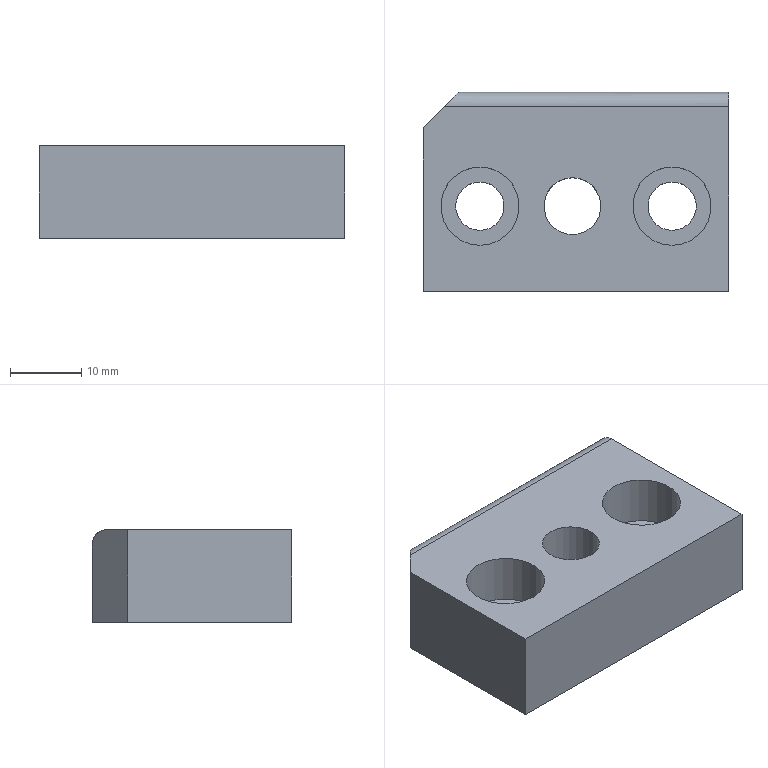Part | STEP file | gslz 2016.10.28-13_id298_x_t | 1 solid | 15 faces | box 43 x 28 x 13 mm | volume 13037 mm3 | plane 9 | cylinder 6 | commonest cylinder face diameters 6.8 x2 11 x2 4 x1 8 x1
STEP:
#1=CARTESIAN_POINT('',(0.,0.,0.));
#2=DIRECTION('',(0.,0.,1.));
#3=DIRECTION('',(1.,0.,0.));
#4=AXIS2_PLACEMENT_3D('',#1,#2,#3);
#5=CARTESIAN_POINT('',(72.5,53.692,-13.));
#6=VERTEX_POINT('',#5);
#7=CARTESIAN_POINT('',(72.5,81.692,-13.));
#8=VERTEX_POINT('',#7);
#9=CARTESIAN_POINT('',(72.5,88.142,-13.));
#10=DIRECTION('',(0.,1.,0.));
#11=VECTOR('',#10,1.);
#12=LINE('',#9,#11);
#13=CARTESIAN_POINT('',(72.5,88.142,-5.));
#14=DIRECTION('',(-1.,0.,0.));
#15=DIRECTION('',(0.,0.,-1.));
#16=AXIS2_PLACEMENT_3D('',#13,#14,#15);
#17=PLANE('',#16);
#18=CARTESIAN_POINT('',(8.,0.));
#19=DIRECTION('',(0.,-1.));
#20=VECTOR('',#19,1.);
#21=LINE('',#18,#20);
#22=(GEOMETRIC_REPRESENTATION_CONTEXT(2)PARAMETRIC_REPRESENTATION_CONTEXT()REPRESENTATION_CONTEXT('',''));
#23=DEFINITIONAL_REPRESENTATION('',(#21),#22);
#24=PCURVE('',#17,#23);
#25=CARTESIAN_POINT('',(-412.493,94.567,-13.));
#26=DIRECTION('',(0.,0.,1.));
#27=DIRECTION('',(-1.,0.,0.));
#28=AXIS2_PLACEMENT_3D('',#25,#26,#27);
#29=PLANE('',#28);
#30=CARTESIAN_POINT('',(-484.993,6.425));
#31=DIRECTION('',(0.,-1.));
#32=VECTOR('',#31,1.);
#33=LINE('',#30,#32);
#34=(GEOMETRIC_REPRESENTATION_CONTEXT(2)PARAMETRIC_REPRESENTATION_CONTEXT()REPRESENTATION_CONTEXT('',''));
#35=DEFINITIONAL_REPRESENTATION('',(#33),#34);
#36=PCURVE('',#29,#35);
#37=SURFACE_CURVE('',#12,(#24,#36),.PCURVE_S1.);
#38=EDGE_CURVE('',#6,#8,#37,.T.);
#39=ORIENTED_EDGE('',*,*,#38,.T.);
#40=CARTESIAN_POINT('',(72.5,81.692,-2.));
#41=VERTEX_POINT('',#40);
#42=CARTESIAN_POINT('',(72.5,81.692,-5.));
#43=DIRECTION('',(0.,0.,1.));
#44=VECTOR('',#43,1.);
#45=LINE('',#42,#44);
#46=CARTESIAN_POINT('',(0.,6.45));
#47=DIRECTION('',(-1.,0.));
#48=VECTOR('',#47,1.);
#49=LINE('',#46,#48);
#50=(GEOMETRIC_REPRESENTATION_CONTEXT(2)PARAMETRIC_REPRESENTATION_CONTEXT()REPRESENTATION_CONTEXT('',''));
#51=DEFINITIONAL_REPRESENTATION('',(#49),#50);
#52=PCURVE('',#17,#51);
#53=CARTESIAN_POINT('',(-39.228,81.692,-16.));
#54=DIRECTION('',(0.,-1.,0.));
#55=DIRECTION('',(0.,0.,1.));
#56=AXIS2_PLACEMENT_3D('',#53,#54,#55);
#57=PLANE('',#56);
#58=CARTESIAN_POINT('',(11.,-111.728));
#59=DIRECTION('',(1.,0.));
#60=VECTOR('',#59,1.);
#61=LINE('',#58,#60);
#62=(GEOMETRIC_REPRESENTATION_CONTEXT(2)PARAMETRIC_REPRESENTATION_CONTEXT()REPRESENTATION_CONTEXT('',''));
#63=DEFINITIONAL_REPRESENTATION('',(#61),#62);
#64=PCURVE('',#57,#63);
#65=SURFACE_CURVE('',#45,(#52,#64),.PCURVE_S1.);
#66=EDGE_CURVE('',#8,#41,#65,.T.);
#67=ORIENTED_EDGE('',*,*,#66,.T.);
#68=CARTESIAN_POINT('',(72.5,79.692,0.));
#69=VERTEX_POINT('',#68);
#70=CARTESIAN_POINT('',(72.5,79.692,-2.));
#71=DIRECTION('',(-1.,0.,0.));
#72=DIRECTION('',(0.,0.,1.));
#73=AXIS2_PLACEMENT_3D('',#70,#71,#72);
#74=CIRCLE('',#73,2.);
#75=CARTESIAN_POINT('',(-3.,8.45));
#76=DIRECTION('',(-1.,0.));
#77=AXIS2_PLACEMENT_2D('',#75,#76);
#78=CIRCLE('',#77,2.);
#79=(GEOMETRIC_REPRESENTATION_CONTEXT(2)PARAMETRIC_REPRESENTATION_CONTEXT()REPRESENTATION_CONTEXT('',''));
#80=DEFINITIONAL_REPRESENTATION('',(#78),#79);
#81=PCURVE('',#17,#80);
#82=CARTESIAN_POINT('',(-412.493,79.692,-2.));
#83=DIRECTION('',(1.,0.,0.));
#84=DIRECTION('',(0.,0.,-1.));
#85=AXIS2_PLACEMENT_3D('',#82,#83,#84);
#86=CYLINDRICAL_SURFACE('',#85,2.);
#87=CARTESIAN_POINT('',(3.142,484.993));
#88=DIRECTION('',(-1.,0.));
#89=VECTOR('',#88,1.);
#90=LINE('',#87,#89);
#91=(GEOMETRIC_REPRESENTATION_CONTEXT(2)PARAMETRIC_REPRESENTATION_CONTEXT()REPRESENTATION_CONTEXT('',''));
#92=DEFINITIONAL_REPRESENTATION('',(#90),#91);
#93=PCURVE('',#86,#92);
#94=SURFACE_CURVE('',#74,(#81,#93),.PCURVE_S1.);
#95=EDGE_CURVE('',#69,#41,#94,.T.);
#96=ORIENTED_EDGE('',*,*,#95,.F.);
#97=CARTESIAN_POINT('',(72.5,53.692,0.));
#98=VERTEX_POINT('',#97);
#99=CARTESIAN_POINT('',(72.5,88.142,0.));
#100=DIRECTION('',(0.,-1.,0.));
#101=VECTOR('',#100,1.);
#102=LINE('',#99,#101);
#103=CARTESIAN_POINT('',(-5.,0.));
#104=DIRECTION('',(0.,1.));
#105=VECTOR('',#104,1.);
#106=LINE('',#103,#105);
#107=(GEOMETRIC_REPRESENTATION_CONTEXT(2)PARAMETRIC_REPRESENTATION_CONTEXT()REPRESENTATION_CONTEXT('',''));
#108=DEFINITIONAL_REPRESENTATION('',(#106),#107);
#109=PCURVE('',#17,#108);
#110=CARTESIAN_POINT('',(-412.493,94.567,0.));
#111=DIRECTION('',(0.,0.,1.));
#112=DIRECTION('',(-1.,0.,0.));
#113=AXIS2_PLACEMENT_3D('',#110,#111,#112);
#114=PLANE('',#113);
#115=CARTESIAN_POINT('',(-484.993,6.425));
#116=DIRECTION('',(0.,1.));
#117=VECTOR('',#116,1.);
#118=LINE('',#115,#117);
#119=(GEOMETRIC_REPRESENTATION_CONTEXT(2)PARAMETRIC_REPRESENTATION_CONTEXT()REPRESENTATION_CONTEXT('',''));
#120=DEFINITIONAL_REPRESENTATION('',(#118),#119);
#121=PCURVE('',#114,#120);
#122=SURFACE_CURVE('',#102,(#109,#121),.PCURVE_S1.);
#123=EDGE_CURVE('',#69,#98,#122,.T.);
#124=ORIENTED_EDGE('',*,*,#123,.T.);
#125=CARTESIAN_POINT('',(72.5,53.692,-16.));
#126=DIRECTION('',(0.,0.,-1.));
#127=VECTOR('',#126,1.);
#128=LINE('',#125,#127);
#129=CARTESIAN_POINT('',(11.,34.45));
#130=DIRECTION('',(1.,0.));
#131=VECTOR('',#130,1.);
#132=LINE('',#129,#131);
#133=(GEOMETRIC_REPRESENTATION_CONTEXT(2)PARAMETRIC_REPRESENTATION_CONTEXT()REPRESENTATION_CONTEXT('',''));
#134=DEFINITIONAL_REPRESENTATION('',(#132),#133);
#135=PCURVE('',#17,#134);
#136=CARTESIAN_POINT('',(-39.228,53.692,-16.));
#137=DIRECTION('',(0.,-1.,0.));
#138=DIRECTION('',(0.,0.,1.));
#139=AXIS2_PLACEMENT_3D('',#136,#137,#138);
#140=PLANE('',#139);
#141=CARTESIAN_POINT('',(0.,-111.728));
#142=DIRECTION('',(-1.,0.));
#143=VECTOR('',#142,1.);
#144=LINE('',#141,#143);
#145=(GEOMETRIC_REPRESENTATION_CONTEXT(2)PARAMETRIC_REPRESENTATION_CONTEXT()REPRESENTATION_CONTEXT('',''));
#146=DEFINITIONAL_REPRESENTATION('',(#144),#145);
#147=PCURVE('',#140,#146);
#148=SURFACE_CURVE('',#128,(#135,#147),.PCURVE_S1.);
#149=EDGE_CURVE('',#98,#6,#148,.T.);
#150=ORIENTED_EDGE('',*,*,#149,.T.);
#151=EDGE_LOOP('',(#39,#67,#96,#124,#150));
#152=FACE_BOUND('',#151,.T.);
#153=ADVANCED_FACE('',(#152),#17,.F.);
#154=CARTESIAN_POINT('',(29.5,53.692,0.));
#155=VERTEX_POINT('',#154);
#156=CARTESIAN_POINT('',(29.5,76.692,0.));
#157=VERTEX_POINT('',#156);
#158=CARTESIAN_POINT('',(29.5,88.142,0.));
#159=DIRECTION('',(0.,1.,0.));
#160=VECTOR('',#159,1.);
#161=LINE('',#158,#160);
#162=CARTESIAN_POINT('',(29.5,88.142,-5.));
#163=DIRECTION('',(-1.,0.,0.));
#164=DIRECTION('',(0.,0.,-1.));
#165=AXIS2_PLACEMENT_3D('',#162,#163,#164);
#166=PLANE('',#165);
#167=CARTESIAN_POINT('',(-5.,0.));
#168=DIRECTION('',(0.,-1.));
#169=VECTOR('',#168,1.);
#170=LINE('',#167,#169);
#171=(GEOMETRIC_REPRESENTATION_CONTEXT(2)PARAMETRIC_REPRESENTATION_CONTEXT()REPRESENTATION_CONTEXT('',''));
#172=DEFINITIONAL_REPRESENTATION('',(#170),#171);
#173=PCURVE('',#166,#172);
#174=CARTESIAN_POINT('',(-441.993,6.425));
#175=DIRECTION('',(0.,-1.));
#176=VECTOR('',#175,1.);
#177=LINE('',#174,#176);
#178=(GEOMETRIC_REPRESENTATION_CONTEXT(2)PARAMETRIC_REPRESENTATION_CONTEXT()REPRESENTATION_CONTEXT('',''));
#179=DEFINITIONAL_REPRESENTATION('',(#177),#178);
#180=PCURVE('',#114,#179);
#181=SURFACE_CURVE('',#161,(#173,#180),.PCURVE_S1.);
#182=EDGE_CURVE('',#155,#157,#181,.T.);
#183=ORIENTED_EDGE('',*,*,#182,.T.);
#184=CARTESIAN_POINT('',(29.5,76.692,-13.));
#185=VERTEX_POINT('',#184);
#186=CARTESIAN_POINT('',(29.5,76.692,-5.));
#187=DIRECTION('',(0.,0.,-1.));
#188=VECTOR('',#187,1.);
#189=LINE('',#186,#188);
#190=CARTESIAN_POINT('',(0.,11.45));
#191=DIRECTION('',(1.,0.));
#192=VECTOR('',#191,1.);
#193=LINE('',#190,#192);
#194=(GEOMETRIC_REPRESENTATION_CONTEXT(2)PARAMETRIC_REPRESENTATION_CONTEXT()REPRESENTATION_CONTEXT('',''));
#195=DEFINITIONAL_REPRESENTATION('',(#193),#194);
#196=PCURVE('',#166,#195);
#197=CARTESIAN_POINT('',(34.5,81.692,-16.));
#198=DIRECTION('',(-0.7071,0.7071,0.));
#199=DIRECTION('',(-0.7071,-0.7071,0.));
#200=AXIS2_PLACEMENT_3D('',#197,#198,#199);
#201=PLANE('',#200);
#202=CARTESIAN_POINT('',(7.071,11.));
#203=DIRECTION('',(0.,-1.));
#204=VECTOR('',#203,1.);
#205=LINE('',#202,#204);
#206=(GEOMETRIC_REPRESENTATION_CONTEXT(2)PARAMETRIC_REPRESENTATION_CONTEXT()REPRESENTATION_CONTEXT('',''));
#207=DEFINITIONAL_REPRESENTATION('',(#205),#206);
#208=PCURVE('',#201,#207);
#209=SURFACE_CURVE('',#189,(#196,#208),.PCURVE_S1.);
#210=EDGE_CURVE('',#157,#185,#209,.T.);
#211=ORIENTED_EDGE('',*,*,#210,.T.);
#212=CARTESIAN_POINT('',(29.5,53.692,-13.));
#213=VERTEX_POINT('',#212);
#214=CARTESIAN_POINT('',(29.5,88.142,-13.));
#215=DIRECTION('',(0.,-1.,0.));
#216=VECTOR('',#215,1.);
#217=LINE('',#214,#216);
#218=CARTESIAN_POINT('',(8.,0.));
#219=DIRECTION('',(0.,1.));
#220=VECTOR('',#219,1.);
#221=LINE('',#218,#220);
#222=(GEOMETRIC_REPRESENTATION_CONTEXT(2)PARAMETRIC_REPRESENTATION_CONTEXT()REPRESENTATION_CONTEXT('',''));
#223=DEFINITIONAL_REPRESENTATION('',(#221),#222);
#224=PCURVE('',#166,#223);
#225=CARTESIAN_POINT('',(-441.993,6.425));
#226=DIRECTION('',(0.,1.));
#227=VECTOR('',#226,1.);
#228=LINE('',#225,#227);
#229=(GEOMETRIC_REPRESENTATION_CONTEXT(2)PARAMETRIC_REPRESENTATION_CONTEXT()REPRESENTATION_CONTEXT('',''));
#230=DEFINITIONAL_REPRESENTATION('',(#228),#229);
#231=PCURVE('',#29,#230);
#232=SURFACE_CURVE('',#217,(#224,#231),.PCURVE_S1.);
#233=EDGE_CURVE('',#185,#213,#232,.T.);
#234=ORIENTED_EDGE('',*,*,#233,.T.);
#235=CARTESIAN_POINT('',(29.5,53.692,-5.));
#236=DIRECTION('',(0.,0.,-1.));
#237=VECTOR('',#236,1.);
#238=LINE('',#235,#237);
#239=CARTESIAN_POINT('',(0.,34.45));
#240=DIRECTION('',(1.,0.));
#241=VECTOR('',#240,1.);
#242=LINE('',#239,#241);
#243=(GEOMETRIC_REPRESENTATION_CONTEXT(2)PARAMETRIC_REPRESENTATION_CONTEXT()REPRESENTATION_CONTEXT('',''));
#244=DEFINITIONAL_REPRESENTATION('',(#242),#243);
#245=PCURVE('',#166,#244);
#246=CARTESIAN_POINT('',(11.,-68.728));
#247=DIRECTION('',(-1.,0.));
#248=VECTOR('',#247,1.);
#249=LINE('',#246,#248);
#250=(GEOMETRIC_REPRESENTATION_CONTEXT(2)PARAMETRIC_REPRESENTATION_CONTEXT()REPRESENTATION_CONTEXT('',''));
#251=DEFINITIONAL_REPRESENTATION('',(#249),#250);
#252=PCURVE('',#140,#251);
#253=SURFACE_CURVE('',#238,(#245,#252),.PCURVE_S1.);
#254=EDGE_CURVE('',#155,#213,#253,.T.);
#255=ORIENTED_EDGE('',*,*,#254,.F.);
#256=EDGE_LOOP('',(#183,#211,#234,#255));
#257=FACE_BOUND('',#256,.T.);
#258=ADVANCED_FACE('',(#257),#166,.T.);
#259=CARTESIAN_POINT('',(64.5,60.192,0.));
#260=VERTEX_POINT('',#259);
#261=CARTESIAN_POINT('',(64.5,65.692,0.));
#262=DIRECTION('',(0.,0.,-1.));
#263=DIRECTION('',(0.,-1.,0.));
#264=AXIS2_PLACEMENT_3D('',#261,#262,#263);
#265=CIRCLE('',#264,5.5);
#266=CARTESIAN_POINT('',(-476.993,34.375));
#267=CARTESIAN_POINT('',(-467.467,34.375));
#268=CARTESIAN_POINT('',(-472.23,26.125));
#269=CARTESIAN_POINT('',(-476.993,17.875));
#270=CARTESIAN_POINT('',(-481.756,26.125));
#271=CARTESIAN_POINT('',(-486.519,34.375));
#272=CARTESIAN_POINT('',(-476.993,34.375));
#273=(BOUNDED_CURVE()B_SPLINE_CURVE(2,(#266,#267,#268,#269,#270,#271,#272),.UNSPECIFIED.,.T.,.F.)B_SPLINE_CURVE_WITH_KNOTS((1,2,2,2,2,1),(-2.094,0.,2.094,4.189,6.283,8.378),.UNSPECIFIED.)CURVE()GEOMETRIC_REPRESENTATION_ITEM()RATIONAL_B_SPLINE_CURVE((1.,0.5,1.,0.5,1.,0.5,1.))REPRESENTATION_ITEM(''));
#274=(GEOMETRIC_REPRESENTATION_CONTEXT(2)PARAMETRIC_REPRESENTATION_CONTEXT()REPRESENTATION_CONTEXT('',''));
#275=DEFINITIONAL_REPRESENTATION('',(#273),#274);
#276=PCURVE('',#114,#275);
#277=CARTESIAN_POINT('',(64.5,65.692,0.));
#278=DIRECTION('',(0.,0.,-1.));
#279=DIRECTION('',(0.,-1.,0.));
#280=AXIS2_PLACEMENT_3D('',#277,#278,#279);
#281=CYLINDRICAL_SURFACE('',#280,5.5);
#282=CARTESIAN_POINT('',(0.,0.));
#283=DIRECTION('',(1.,0.));
#284=VECTOR('',#283,1.);
#285=LINE('',#282,#284);
#286=(GEOMETRIC_REPRESENTATION_CONTEXT(2)PARAMETRIC_REPRESENTATION_CONTEXT()REPRESENTATION_CONTEXT('',''));
#287=DEFINITIONAL_REPRESENTATION('',(#285),#286);
#288=PCURVE('',#281,#287);
#289=SURFACE_CURVE('',#265,(#276,#288),.PCURVE_S1.);
#290=EDGE_CURVE('',#260,#260,#289,.T.);
#291=ORIENTED_EDGE('',*,*,#290,.T.);
#292=EDGE_LOOP('',(#291));
#293=FACE_BOUND('',#292,.T.);
#294=CARTESIAN_POINT('',(37.5,60.192,0.));
#295=VERTEX_POINT('',#294);
#296=CARTESIAN_POINT('',(37.5,65.692,0.));
#297=DIRECTION('',(0.,0.,-1.));
#298=DIRECTION('',(0.,-1.,0.));
#299=AXIS2_PLACEMENT_3D('',#296,#297,#298);
#300=CIRCLE('',#299,5.5);
#301=CARTESIAN_POINT('',(-449.993,34.375));
#302=CARTESIAN_POINT('',(-440.467,34.375));
#303=CARTESIAN_POINT('',(-445.23,26.125));
#304=CARTESIAN_POINT('',(-449.993,17.875));
#305=CARTESIAN_POINT('',(-454.756,26.125));
#306=CARTESIAN_POINT('',(-459.519,34.375));
#307=CARTESIAN_POINT('',(-449.993,34.375));
#308=(BOUNDED_CURVE()B_SPLINE_CURVE(2,(#301,#302,#303,#304,#305,#306,#307),.UNSPECIFIED.,.T.,.F.)B_SPLINE_CURVE_WITH_KNOTS((1,2,2,2,2,1),(-2.094,0.,2.094,4.189,6.283,8.378),.UNSPECIFIED.)CURVE()GEOMETRIC_REPRESENTATION_ITEM()RATIONAL_B_SPLINE_CURVE((1.,0.5,1.,0.5,1.,0.5,1.))REPRESENTATION_ITEM(''));
#309=(GEOMETRIC_REPRESENTATION_CONTEXT(2)PARAMETRIC_REPRESENTATION_CONTEXT()REPRESENTATION_CONTEXT('',''));
#310=DEFINITIONAL_REPRESENTATION('',(#308),#309);
#311=PCURVE('',#114,#310);
#312=CARTESIAN_POINT('',(37.5,65.692,0.));
#313=DIRECTION('',(0.,0.,-1.));
#314=DIRECTION('',(0.,-1.,0.));
#315=AXIS2_PLACEMENT_3D('',#312,#313,#314);
#316=CYLINDRICAL_SURFACE('',#315,5.5);
#317=CARTESIAN_POINT('',(0.,0.));
#318=DIRECTION('',(1.,0.));
#319=VECTOR('',#318,1.);
#320=LINE('',#317,#319);
#321=(GEOMETRIC_REPRESENTATION_CONTEXT(2)PARAMETRIC_REPRESENTATION_CONTEXT()REPRESENTATION_CONTEXT('',''));
#322=DEFINITIONAL_REPRESENTATION('',(#320),#321);
#323=PCURVE('',#316,#322);
#324=SURFACE_CURVE('',#300,(#311,#323),.PCURVE_S1.);
#325=EDGE_CURVE('',#295,#295,#324,.T.);
#326=ORIENTED_EDGE('',*,*,#325,.T.);
#327=EDGE_LOOP('',(#326));
#328=FACE_BOUND('',#327,.T.);
#329=CARTESIAN_POINT('',(50.5,61.692,0.));
#330=VERTEX_POINT('',#329);
#331=CARTESIAN_POINT('',(50.5,65.692,0.));
#332=DIRECTION('',(0.,0.,1.));
#333=DIRECTION('',(0.,-1.,0.));
#334=AXIS2_PLACEMENT_3D('',#331,#332,#333);
#335=CIRCLE('',#334,4.);
#336=CARTESIAN_POINT('',(-462.993,28.875));
#337=DIRECTION('',(0.,1.));
#338=AXIS2_PLACEMENT_2D('',#336,#337);
#339=CIRCLE('',#338,4.);
#340=(GEOMETRIC_REPRESENTATION_CONTEXT(2)PARAMETRIC_REPRESENTATION_CONTEXT()REPRESENTATION_CONTEXT('',''));
#341=DEFINITIONAL_REPRESENTATION('',(#339),#340);
#342=PCURVE('',#114,#341);
#343=CARTESIAN_POINT('',(50.5,65.692,-50.));
#344=DIRECTION('',(0.,0.,-1.));
#345=DIRECTION('',(0.,-1.,0.));
#346=AXIS2_PLACEMENT_3D('',#343,#344,#345);
#347=CYLINDRICAL_SURFACE('',#346,4.);
#348=CARTESIAN_POINT('',(6.283,-50.));
#349=DIRECTION('',(-1.,0.));
#350=VECTOR('',#349,1.);
#351=LINE('',#348,#350);
#352=(GEOMETRIC_REPRESENTATION_CONTEXT(2)PARAMETRIC_REPRESENTATION_CONTEXT()REPRESENTATION_CONTEXT('',''));
#353=DEFINITIONAL_REPRESENTATION('',(#351),#352);
#354=PCURVE('',#347,#353);
#355=SURFACE_CURVE('',#335,(#342,#354),.PCURVE_S1.);
#356=EDGE_CURVE('',#330,#330,#355,.T.);
#357=ORIENTED_EDGE('',*,*,#356,.F.);
#358=EDGE_LOOP('',(#357));
#359=FACE_BOUND('',#358,.T.);
#360=ORIENTED_EDGE('',*,*,#123,.F.);
#361=CARTESIAN_POINT('',(32.5,79.692,0.));
#362=VERTEX_POINT('',#361);
#363=CARTESIAN_POINT('',(-412.493,79.692,0.));
#364=DIRECTION('',(-1.,0.,0.));
#365=VECTOR('',#364,1.);
#366=LINE('',#363,#365);
#367=CARTESIAN_POINT('',(0.,14.875));
#368=DIRECTION('',(1.,0.));
#369=VECTOR('',#368,1.);
#370=LINE('',#367,#369);
#371=(GEOMETRIC_REPRESENTATION_CONTEXT(2)PARAMETRIC_REPRESENTATION_CONTEXT()REPRESENTATION_CONTEXT('',''));
#372=DEFINITIONAL_REPRESENTATION('',(#370),#371);
#373=PCURVE('',#114,#372);
#374=CARTESIAN_POINT('',(3.142,0.));
#375=DIRECTION('',(0.,-1.));
#376=VECTOR('',#375,1.);
#377=LINE('',#374,#376);
#378=(GEOMETRIC_REPRESENTATION_CONTEXT(2)PARAMETRIC_REPRESENTATION_CONTEXT()REPRESENTATION_CONTEXT('',''));
#379=DEFINITIONAL_REPRESENTATION('',(#377),#378);
#380=PCURVE('',#86,#379);
#381=SURFACE_CURVE('',#366,(#373,#380),.PCURVE_S1.);
#382=EDGE_CURVE('',#69,#362,#381,.T.);
#383=ORIENTED_EDGE('',*,*,#382,.T.);
#384=CARTESIAN_POINT('',(-182.559,-135.367,0.));
#385=DIRECTION('',(-0.7071,-0.7071,0.));
#386=VECTOR('',#385,1.);
#387=LINE('',#384,#386);
#388=CARTESIAN_POINT('',(-229.934,229.934));
#389=DIRECTION('',(0.7071,0.7071));
#390=VECTOR('',#389,1.);
#391=LINE('',#388,#390);
#392=(GEOMETRIC_REPRESENTATION_CONTEXT(2)PARAMETRIC_REPRESENTATION_CONTEXT()REPRESENTATION_CONTEXT('',''));
#393=DEFINITIONAL_REPRESENTATION('',(#391),#392);
#394=PCURVE('',#114,#393);
#395=CARTESIAN_POINT('',(306.968,16.));
#396=DIRECTION('',(1.,0.));
#397=VECTOR('',#396,1.);
#398=LINE('',#395,#397);
#399=(GEOMETRIC_REPRESENTATION_CONTEXT(2)PARAMETRIC_REPRESENTATION_CONTEXT()REPRESENTATION_CONTEXT('',''));
#400=DEFINITIONAL_REPRESENTATION('',(#398),#399);
#401=PCURVE('',#201,#400);
#402=SURFACE_CURVE('',#387,(#394,#401),.PCURVE_S1.);
#403=EDGE_CURVE('',#362,#157,#402,.T.);
#404=ORIENTED_EDGE('',*,*,#403,.T.);
#405=ORIENTED_EDGE('',*,*,#182,.F.);
#406=CARTESIAN_POINT('',(-39.228,53.692,0.));
#407=DIRECTION('',(-1.,0.,0.));
#408=VECTOR('',#407,1.);
#409=LINE('',#406,#408);
#410=CARTESIAN_POINT('',(-373.265,40.875));
#411=DIRECTION('',(1.,0.));
#412=VECTOR('',#411,1.);
#413=LINE('',#410,#412);
#414=(GEOMETRIC_REPRESENTATION_CONTEXT(2)PARAMETRIC_REPRESENTATION_CONTEXT()REPRESENTATION_CONTEXT('',''));
#415=DEFINITIONAL_REPRESENTATION('',(#413),#414);
#416=PCURVE('',#114,#415);
#417=CARTESIAN_POINT('',(16.,0.));
#418=DIRECTION('',(0.,1.));
#419=VECTOR('',#418,1.);
#420=LINE('',#417,#419);
#421=(GEOMETRIC_REPRESENTATION_CONTEXT(2)PARAMETRIC_REPRESENTATION_CONTEXT()REPRESENTATION_CONTEXT('',''));
#422=DEFINITIONAL_REPRESENTATION('',(#420),#421);
#423=PCURVE('',#140,#422);
#424=SURFACE_CURVE('',#409,(#416,#423),.PCURVE_S1.);
#425=EDGE_CURVE('',#98,#155,#424,.T.);
#426=ORIENTED_EDGE('',*,*,#425,.F.);
#427=EDGE_LOOP('',(#360,#383,#404,#405,#426));
#428=FACE_BOUND('',#427,.T.);
#429=ADVANCED_FACE('',(#293,#328,#359,#428),#114,.T.);
#430=CARTESIAN_POINT('',(64.5,62.292,-13.));
#431=VERTEX_POINT('',#430);
#432=CARTESIAN_POINT('',(64.5,65.692,-13.));
#433=DIRECTION('',(0.,0.,-1.));
#434=DIRECTION('',(0.,-1.,0.));
#435=AXIS2_PLACEMENT_3D('',#432,#433,#434);
#436=CIRCLE('',#435,3.4);
#437=CARTESIAN_POINT('',(-476.993,32.275));
#438=CARTESIAN_POINT('',(-471.104,32.275));
#439=CARTESIAN_POINT('',(-474.048,27.175));
#440=CARTESIAN_POINT('',(-476.993,22.075));
#441=CARTESIAN_POINT('',(-479.937,27.175));
#442=CARTESIAN_POINT('',(-482.882,32.275));
#443=CARTESIAN_POINT('',(-476.993,32.275));
#444=(BOUNDED_CURVE()B_SPLINE_CURVE(2,(#437,#438,#439,#440,#441,#442,#443),.UNSPECIFIED.,.T.,.F.)B_SPLINE_CURVE_WITH_KNOTS((1,2,2,2,2,1),(-2.094,0.,2.094,4.189,6.283,8.378),.UNSPECIFIED.)CURVE()GEOMETRIC_REPRESENTATION_ITEM()RATIONAL_B_SPLINE_CURVE((1.,0.5,1.,0.5,1.,0.5,1.))REPRESENTATION_ITEM(''));
#445=(GEOMETRIC_REPRESENTATION_CONTEXT(2)PARAMETRIC_REPRESENTATION_CONTEXT()REPRESENTATION_CONTEXT('',''));
#446=DEFINITIONAL_REPRESENTATION('',(#444),#445);
#447=PCURVE('',#29,#446);
#448=CARTESIAN_POINT('',(64.5,65.692,-50.));
#449=DIRECTION('',(0.,0.,-1.));
#450=DIRECTION('',(0.,-1.,0.));
#451=AXIS2_PLACEMENT_3D('',#448,#449,#450);
#452=CYLINDRICAL_SURFACE('',#451,3.4);
#453=CARTESIAN_POINT('',(0.,-37.));
#454=DIRECTION('',(1.,0.));
#455=VECTOR('',#454,1.);
#456=LINE('',#453,#455);
#457=(GEOMETRIC_REPRESENTATION_CONTEXT(2)PARAMETRIC_REPRESENTATION_CONTEXT()REPRESENTATION_CONTEXT('',''));
#458=DEFINITIONAL_REPRESENTATION('',(#456),#457);
#459=PCURVE('',#452,#458);
#460=SURFACE_CURVE('',#436,(#447,#459),.PCURVE_S1.);
#461=EDGE_CURVE('',#431,#431,#460,.T.);
#462=ORIENTED_EDGE('',*,*,#461,.F.);
#463=EDGE_LOOP('',(#462));
#464=FACE_BOUND('',#463,.T.);
#465=CARTESIAN_POINT('',(37.5,62.292,-13.));
#466=VERTEX_POINT('',#465);
#467=CARTESIAN_POINT('',(37.5,65.692,-13.));
#468=DIRECTION('',(0.,0.,-1.));
#469=DIRECTION('',(0.,-1.,0.));
#470=AXIS2_PLACEMENT_3D('',#467,#468,#469);
#471=CIRCLE('',#470,3.4);
#472=CARTESIAN_POINT('',(-449.993,32.275));
#473=CARTESIAN_POINT('',(-444.104,32.275));
#474=CARTESIAN_POINT('',(-447.048,27.175));
#475=CARTESIAN_POINT('',(-449.993,22.075));
#476=CARTESIAN_POINT('',(-452.937,27.175));
#477=CARTESIAN_POINT('',(-455.882,32.275));
#478=CARTESIAN_POINT('',(-449.993,32.275));
#479=(BOUNDED_CURVE()B_SPLINE_CURVE(2,(#472,#473,#474,#475,#476,#477,#478),.UNSPECIFIED.,.T.,.F.)B_SPLINE_CURVE_WITH_KNOTS((1,2,2,2,2,1),(-2.094,0.,2.094,4.189,6.283,8.378),.UNSPECIFIED.)CURVE()GEOMETRIC_REPRESENTATION_ITEM()RATIONAL_B_SPLINE_CURVE((1.,0.5,1.,0.5,1.,0.5,1.))REPRESENTATION_ITEM(''));
#480=(GEOMETRIC_REPRESENTATION_CONTEXT(2)PARAMETRIC_REPRESENTATION_CONTEXT()REPRESENTATION_CONTEXT('',''));
#481=DEFINITIONAL_REPRESENTATION('',(#479),#480);
#482=PCURVE('',#29,#481);
#483=CARTESIAN_POINT('',(37.5,65.692,-50.));
#484=DIRECTION('',(0.,0.,-1.));
#485=DIRECTION('',(0.,-1.,0.));
#486=AXIS2_PLACEMENT_3D('',#483,#484,#485);
#487=CYLINDRICAL_SURFACE('',#486,3.4);
#488=CARTESIAN_POINT('',(0.,-37.));
#489=DIRECTION('',(1.,0.));
#490=VECTOR('',#489,1.);
#491=LINE('',#488,#490);
#492=(GEOMETRIC_REPRESENTATION_CONTEXT(2)PARAMETRIC_REPRESENTATION_CONTEXT()REPRESENTATION_CONTEXT('',''));
#493=DEFINITIONAL_REPRESENTATION('',(#491),#492);
#494=PCURVE('',#487,#493);
#495=SURFACE_CURVE('',#471,(#482,#494),.PCURVE_S1.);
#496=EDGE_CURVE('',#466,#466,#495,.T.);
#497=ORIENTED_EDGE('',*,*,#496,.F.);
#498=EDGE_LOOP('',(#497));
#499=FACE_BOUND('',#498,.T.);
#500=CARTESIAN_POINT('',(50.5,61.692,-13.));
#501=VERTEX_POINT('',#500);
#502=CARTESIAN_POINT('',(50.5,65.692,-13.));
#503=DIRECTION('',(0.,0.,-1.));
#504=DIRECTION('',(0.,-1.,0.));
#505=AXIS2_PLACEMENT_3D('',#502,#503,#504);
#506=CIRCLE('',#505,4.);
#507=CARTESIAN_POINT('',(-462.993,32.875));
#508=CARTESIAN_POINT('',(-456.065,32.875));
#509=CARTESIAN_POINT('',(-459.529,26.875));
#510=CARTESIAN_POINT('',(-462.993,20.875));
#511=CARTESIAN_POINT('',(-466.457,26.875));
#512=CARTESIAN_POINT('',(-469.921,32.875));
#513=CARTESIAN_POINT('',(-462.993,32.875));
#514=(BOUNDED_CURVE()B_SPLINE_CURVE(2,(#507,#508,#509,#510,#511,#512,#513),.UNSPECIFIED.,.T.,.F.)B_SPLINE_CURVE_WITH_KNOTS((1,2,2,2,2,1),(-2.094,0.,2.094,4.189,6.283,8.378),.UNSPECIFIED.)CURVE()GEOMETRIC_REPRESENTATION_ITEM()RATIONAL_B_SPLINE_CURVE((1.,0.5,1.,0.5,1.,0.5,1.))REPRESENTATION_ITEM(''));
#515=(GEOMETRIC_REPRESENTATION_CONTEXT(2)PARAMETRIC_REPRESENTATION_CONTEXT()REPRESENTATION_CONTEXT('',''));
#516=DEFINITIONAL_REPRESENTATION('',(#514),#515);
#517=PCURVE('',#29,#516);
#518=CARTESIAN_POINT('',(0.,-37.));
#519=DIRECTION('',(1.,0.));
#520=VECTOR('',#519,1.);
#521=LINE('',#518,#520);
#522=(GEOMETRIC_REPRESENTATION_CONTEXT(2)PARAMETRIC_REPRESENTATION_CONTEXT()REPRESENTATION_CONTEXT('',''));
#523=DEFINITIONAL_REPRESENTATION('',(#521),#522);
#524=PCURVE('',#347,#523);
#525=SURFACE_CURVE('',#506,(#517,#524),.PCURVE_S1.);
#526=EDGE_CURVE('',#501,#501,#525,.T.);
#527=ORIENTED_EDGE('',*,*,#526,.F.);
#528=EDGE_LOOP('',(#527));
#529=FACE_BOUND('',#528,.T.);
#530=ORIENTED_EDGE('',*,*,#233,.F.);
#531=CARTESIAN_POINT('',(34.5,81.692,-13.));
#532=VERTEX_POINT('',#531);
#533=CARTESIAN_POINT('',(-182.559,-135.367,-13.));
#534=DIRECTION('',(0.7071,0.7071,0.));
#535=VECTOR('',#534,1.);
#536=LINE('',#533,#535);
#537=CARTESIAN_POINT('',(-229.934,229.934));
#538=DIRECTION('',(-0.7071,-0.7071));
#539=VECTOR('',#538,1.);
#540=LINE('',#537,#539);
#541=(GEOMETRIC_REPRESENTATION_CONTEXT(2)PARAMETRIC_REPRESENTATION_CONTEXT()REPRESENTATION_CONTEXT('',''));
#542=DEFINITIONAL_REPRESENTATION('',(#540),#541);
#543=PCURVE('',#29,#542);
#544=CARTESIAN_POINT('',(306.968,3.));
#545=DIRECTION('',(-1.,0.));
#546=VECTOR('',#545,1.);
#547=LINE('',#544,#546);
#548=(GEOMETRIC_REPRESENTATION_CONTEXT(2)PARAMETRIC_REPRESENTATION_CONTEXT()REPRESENTATION_CONTEXT('',''));
#549=DEFINITIONAL_REPRESENTATION('',(#547),#548);
#550=PCURVE('',#201,#549);
#551=SURFACE_CURVE('',#536,(#543,#550),.PCURVE_S1.);
#552=EDGE_CURVE('',#185,#532,#551,.T.);
#553=ORIENTED_EDGE('',*,*,#552,.T.);
#554=CARTESIAN_POINT('',(-39.228,81.692,-13.));
#555=DIRECTION('',(-1.,0.,0.));
#556=VECTOR('',#555,1.);
#557=LINE('',#554,#556);
#558=CARTESIAN_POINT('',(-373.265,12.875));
#559=DIRECTION('',(1.,0.));
#560=VECTOR('',#559,1.);
#561=LINE('',#558,#560);
#562=(GEOMETRIC_REPRESENTATION_CONTEXT(2)PARAMETRIC_REPRESENTATION_CONTEXT()REPRESENTATION_CONTEXT('',''));
#563=DEFINITIONAL_REPRESENTATION('',(#561),#562);
#564=PCURVE('',#29,#563);
#565=CARTESIAN_POINT('',(3.,0.));
#566=DIRECTION('',(0.,1.));
#567=VECTOR('',#566,1.);
#568=LINE('',#565,#567);
#569=(GEOMETRIC_REPRESENTATION_CONTEXT(2)PARAMETRIC_REPRESENTATION_CONTEXT()REPRESENTATION_CONTEXT('',''));
#570=DEFINITIONAL_REPRESENTATION('',(#568),#569);
#571=PCURVE('',#57,#570);
#572=SURFACE_CURVE('',#557,(#564,#571),.PCURVE_S1.);
#573=EDGE_CURVE('',#8,#532,#572,.T.);
#574=ORIENTED_EDGE('',*,*,#573,.F.);
#575=ORIENTED_EDGE('',*,*,#38,.F.);
#576=CARTESIAN_POINT('',(-39.228,53.692,-13.));
#577=DIRECTION('',(1.,0.,0.));
#578=VECTOR('',#577,1.);
#579=LINE('',#576,#578);
#580=CARTESIAN_POINT('',(-373.265,40.875));
#581=DIRECTION('',(-1.,0.));
#582=VECTOR('',#581,1.);
#583=LINE('',#580,#582);
#584=(GEOMETRIC_REPRESENTATION_CONTEXT(2)PARAMETRIC_REPRESENTATION_CONTEXT()REPRESENTATION_CONTEXT('',''));
#585=DEFINITIONAL_REPRESENTATION('',(#583),#584);
#586=PCURVE('',#29,#585);
#587=CARTESIAN_POINT('',(3.,0.));
#588=DIRECTION('',(0.,-1.));
#589=VECTOR('',#588,1.);
#590=LINE('',#587,#589);
#591=(GEOMETRIC_REPRESENTATION_CONTEXT(2)PARAMETRIC_REPRESENTATION_CONTEXT()REPRESENTATION_CONTEXT('',''));
#592=DEFINITIONAL_REPRESENTATION('',(#590),#591);
#593=PCURVE('',#140,#592);
#594=SURFACE_CURVE('',#579,(#586,#593),.PCURVE_S1.);
#595=EDGE_CURVE('',#213,#6,#594,.T.);
#596=ORIENTED_EDGE('',*,*,#595,.F.);
#597=EDGE_LOOP('',(#530,#553,#574,#575,#596));
#598=FACE_BOUND('',#597,.T.);
#599=ADVANCED_FACE('',(#464,#499,#529,#598),#29,.F.);
#600=CARTESIAN_POINT('',(64.5,62.292,-7.));
#601=VERTEX_POINT('',#600);
#602=CARTESIAN_POINT('',(64.5,65.692,-7.));
#603=DIRECTION('',(0.,0.,1.));
#604=DIRECTION('',(0.,-1.,0.));
#605=AXIS2_PLACEMENT_3D('',#602,#603,#604);
#606=CIRCLE('',#605,3.4);
#607=CARTESIAN_POINT('',(-412.493,94.567,-7.));
#608=DIRECTION('',(0.,0.,1.));
#609=DIRECTION('',(-1.,0.,0.));
#610=AXIS2_PLACEMENT_3D('',#607,#608,#609);
#611=PLANE('',#610);
#612=CARTESIAN_POINT('',(-476.993,28.875));
#613=DIRECTION('',(0.,1.));
#614=AXIS2_PLACEMENT_2D('',#612,#613);
#615=CIRCLE('',#614,3.4);
#616=(GEOMETRIC_REPRESENTATION_CONTEXT(2)PARAMETRIC_REPRESENTATION_CONTEXT()REPRESENTATION_CONTEXT('',''));
#617=DEFINITIONAL_REPRESENTATION('',(#615),#616);
#618=PCURVE('',#611,#617);
#619=CARTESIAN_POINT('',(6.283,-43.));
#620=DIRECTION('',(-1.,0.));
#621=VECTOR('',#620,1.);
#622=LINE('',#619,#621);
#623=(GEOMETRIC_REPRESENTATION_CONTEXT(2)PARAMETRIC_REPRESENTATION_CONTEXT()REPRESENTATION_CONTEXT('',''));
#624=DEFINITIONAL_REPRESENTATION('',(#622),#623);
#625=PCURVE('',#452,#624);
#626=SURFACE_CURVE('',#606,(#618,#625),.PCURVE_S1.);
#627=EDGE_CURVE('',#601,#601,#626,.T.);
#628=ORIENTED_EDGE('',*,*,#627,.F.);
#629=EDGE_LOOP('',(#628));
#630=FACE_BOUND('',#629,.T.);
#631=CARTESIAN_POINT('',(64.5,60.192,-7.));
#632=VERTEX_POINT('',#631);
#633=CARTESIAN_POINT('',(64.5,65.692,-7.));
#634=DIRECTION('',(0.,0.,1.));
#635=DIRECTION('',(0.,-1.,0.));
#636=AXIS2_PLACEMENT_3D('',#633,#634,#635);
#637=CIRCLE('',#636,5.5);
#638=CARTESIAN_POINT('',(-476.993,28.875));
#639=DIRECTION('',(0.,1.));
#640=AXIS2_PLACEMENT_2D('',#638,#639);
#641=CIRCLE('',#640,5.5);
#642=(GEOMETRIC_REPRESENTATION_CONTEXT(2)PARAMETRIC_REPRESENTATION_CONTEXT()REPRESENTATION_CONTEXT('',''));
#643=DEFINITIONAL_REPRESENTATION('',(#641),#642);
#644=PCURVE('',#611,#643);
#645=CARTESIAN_POINT('',(6.283,7.));
#646=DIRECTION('',(-1.,0.));
#647=VECTOR('',#646,1.);
#648=LINE('',#645,#647);
#649=(GEOMETRIC_REPRESENTATION_CONTEXT(2)PARAMETRIC_REPRESENTATION_CONTEXT()REPRESENTATION_CONTEXT('',''));
#650=DEFINITIONAL_REPRESENTATION('',(#648),#649);
#651=PCURVE('',#281,#650);
#652=SURFACE_CURVE('',#637,(#644,#651),.PCURVE_S1.);
#653=EDGE_CURVE('',#632,#632,#652,.T.);
#654=ORIENTED_EDGE('',*,*,#653,.T.);
#655=EDGE_LOOP('',(#654));
#656=FACE_BOUND('',#655,.T.);
#657=ADVANCED_FACE('',(#630,#656),#611,.T.);
#658=CARTESIAN_POINT('',(37.5,62.292,-7.));
#659=VERTEX_POINT('',#658);
#660=CARTESIAN_POINT('',(37.5,65.692,-7.));
#661=DIRECTION('',(0.,0.,1.));
#662=DIRECTION('',(0.,-1.,0.));
#663=AXIS2_PLACEMENT_3D('',#660,#661,#662);
#664=CIRCLE('',#663,3.4);
#665=CARTESIAN_POINT('',(-412.493,94.567,-7.));
#666=DIRECTION('',(0.,0.,1.));
#667=DIRECTION('',(-1.,0.,0.));
#668=AXIS2_PLACEMENT_3D('',#665,#666,#667);
#669=PLANE('',#668);
#670=CARTESIAN_POINT('',(-449.993,28.875));
#671=DIRECTION('',(0.,1.));
#672=AXIS2_PLACEMENT_2D('',#670,#671);
#673=CIRCLE('',#672,3.4);
#674=(GEOMETRIC_REPRESENTATION_CONTEXT(2)PARAMETRIC_REPRESENTATION_CONTEXT()REPRESENTATION_CONTEXT('',''));
#675=DEFINITIONAL_REPRESENTATION('',(#673),#674);
#676=PCURVE('',#669,#675);
#677=CARTESIAN_POINT('',(6.283,-43.));
#678=DIRECTION('',(-1.,0.));
#679=VECTOR('',#678,1.);
#680=LINE('',#677,#679);
#681=(GEOMETRIC_REPRESENTATION_CONTEXT(2)PARAMETRIC_REPRESENTATION_CONTEXT()REPRESENTATION_CONTEXT('',''));
#682=DEFINITIONAL_REPRESENTATION('',(#680),#681);
#683=PCURVE('',#487,#682);
#684=SURFACE_CURVE('',#664,(#676,#683),.PCURVE_S1.);
#685=EDGE_CURVE('',#659,#659,#684,.T.);
#686=ORIENTED_EDGE('',*,*,#685,.F.);
#687=EDGE_LOOP('',(#686));
#688=FACE_BOUND('',#687,.T.);
#689=CARTESIAN_POINT('',(37.5,60.192,-7.));
#690=VERTEX_POINT('',#689);
#691=CARTESIAN_POINT('',(37.5,65.692,-7.));
#692=DIRECTION('',(0.,0.,1.));
#693=DIRECTION('',(0.,-1.,0.));
#694=AXIS2_PLACEMENT_3D('',#691,#692,#693);
#695=CIRCLE('',#694,5.5);
#696=CARTESIAN_POINT('',(-449.993,28.875));
#697=DIRECTION('',(0.,1.));
#698=AXIS2_PLACEMENT_2D('',#696,#697);
#699=CIRCLE('',#698,5.5);
#700=(GEOMETRIC_REPRESENTATION_CONTEXT(2)PARAMETRIC_REPRESENTATION_CONTEXT()REPRESENTATION_CONTEXT('',''));
#701=DEFINITIONAL_REPRESENTATION('',(#699),#700);
#702=PCURVE('',#669,#701);
#703=CARTESIAN_POINT('',(6.283,7.));
#704=DIRECTION('',(-1.,0.));
#705=VECTOR('',#704,1.);
#706=LINE('',#703,#705);
#707=(GEOMETRIC_REPRESENTATION_CONTEXT(2)PARAMETRIC_REPRESENTATION_CONTEXT()REPRESENTATION_CONTEXT('',''));
#708=DEFINITIONAL_REPRESENTATION('',(#706),#707);
#709=PCURVE('',#316,#708);
#710=SURFACE_CURVE('',#695,(#702,#709),.PCURVE_S1.);
#711=EDGE_CURVE('',#690,#690,#710,.T.);
#712=ORIENTED_EDGE('',*,*,#711,.T.);
#713=EDGE_LOOP('',(#712));
#714=FACE_BOUND('',#713,.T.);
#715=ADVANCED_FACE('',(#688,#714),#669,.T.);
#716=ORIENTED_EDGE('',*,*,#461,.F.);
#717=CARTESIAN_POINT('',(64.5,62.292,-7.));
#718=CARTESIAN_POINT('',(64.5,62.292,-13.));
#719=B_SPLINE_CURVE_WITH_KNOTS('',1,(#717,#718),.UNSPECIFIED.,.F.,.F.,(2,2),(-43.,-37.),.PIECEWISE_BEZIER_KNOTS.);
#720=CARTESIAN_POINT('',(0.,0.));
#721=DIRECTION('',(0.,1.));
#722=VECTOR('',#721,1.);
#723=LINE('',#720,#722);
#724=(GEOMETRIC_REPRESENTATION_CONTEXT(2)PARAMETRIC_REPRESENTATION_CONTEXT()REPRESENTATION_CONTEXT('',''));
#725=DEFINITIONAL_REPRESENTATION('',(#723),#724);
#726=PCURVE('',#452,#725);
#727=CARTESIAN_POINT('',(6.283,0.));
#728=DIRECTION('',(0.,1.));
#729=VECTOR('',#728,1.);
#730=LINE('',#727,#729);
#731=(GEOMETRIC_REPRESENTATION_CONTEXT(2)PARAMETRIC_REPRESENTATION_CONTEXT()REPRESENTATION_CONTEXT('',''));
#732=DEFINITIONAL_REPRESENTATION('',(#730),#731);
#733=PCURVE('',#452,#732);
#734=SEAM_CURVE('',#719,(#726,#733),.PCURVE_S1.);
#735=EDGE_CURVE('',#601,#431,#734,.T.);
#736=ORIENTED_EDGE('',*,*,#735,.F.);
#737=ORIENTED_EDGE('',*,*,#627,.F.);
#738=ORIENTED_EDGE('',*,*,#735,.T.);
#739=EDGE_LOOP('',(#716,#736,#737,#738));
#740=FACE_BOUND('',#739,.F.);
#741=ADVANCED_FACE('',(#740),#452,.F.);
#742=ORIENTED_EDGE('',*,*,#496,.F.);
#743=CARTESIAN_POINT('',(37.5,62.292,-7.));
#744=CARTESIAN_POINT('',(37.5,62.292,-13.));
#745=B_SPLINE_CURVE_WITH_KNOTS('',1,(#743,#744),.UNSPECIFIED.,.F.,.F.,(2,2),(-43.,-37.),.PIECEWISE_BEZIER_KNOTS.);
#746=CARTESIAN_POINT('',(0.,0.));
#747=DIRECTION('',(0.,1.));
#748=VECTOR('',#747,1.);
#749=LINE('',#746,#748);
#750=(GEOMETRIC_REPRESENTATION_CONTEXT(2)PARAMETRIC_REPRESENTATION_CONTEXT()REPRESENTATION_CONTEXT('',''));
#751=DEFINITIONAL_REPRESENTATION('',(#749),#750);
#752=PCURVE('',#487,#751);
#753=CARTESIAN_POINT('',(6.283,0.));
#754=DIRECTION('',(0.,1.));
#755=VECTOR('',#754,1.);
#756=LINE('',#753,#755);
#757=(GEOMETRIC_REPRESENTATION_CONTEXT(2)PARAMETRIC_REPRESENTATION_CONTEXT()REPRESENTATION_CONTEXT('',''));
#758=DEFINITIONAL_REPRESENTATION('',(#756),#757);
#759=PCURVE('',#487,#758);
#760=SEAM_CURVE('',#745,(#752,#759),.PCURVE_S1.);
#761=EDGE_CURVE('',#659,#466,#760,.T.);
#762=ORIENTED_EDGE('',*,*,#761,.F.);
#763=ORIENTED_EDGE('',*,*,#685,.F.);
#764=ORIENTED_EDGE('',*,*,#761,.T.);
#765=EDGE_LOOP('',(#742,#762,#763,#764));
#766=FACE_BOUND('',#765,.F.);
#767=ADVANCED_FACE('',(#766),#487,.F.);
#768=ORIENTED_EDGE('',*,*,#425,.T.);
#769=ORIENTED_EDGE('',*,*,#254,.T.);
#770=ORIENTED_EDGE('',*,*,#595,.T.);
#771=ORIENTED_EDGE('',*,*,#149,.F.);
#772=EDGE_LOOP('',(#768,#769,#770,#771));
#773=FACE_BOUND('',#772,.T.);
#774=ADVANCED_FACE('',(#773),#140,.T.);
#775=ORIENTED_EDGE('',*,*,#653,.T.);
#776=CARTESIAN_POINT('',(64.5,60.192,0.));
#777=CARTESIAN_POINT('',(64.5,60.192,-7.));
#778=B_SPLINE_CURVE_WITH_KNOTS('',1,(#776,#777),.UNSPECIFIED.,.F.,.F.,(2,2),(0.,7.),.PIECEWISE_BEZIER_KNOTS.);
#779=CARTESIAN_POINT('',(0.,0.));
#780=DIRECTION('',(0.,1.));
#781=VECTOR('',#780,1.);
#782=LINE('',#779,#781);
#783=(GEOMETRIC_REPRESENTATION_CONTEXT(2)PARAMETRIC_REPRESENTATION_CONTEXT()REPRESENTATION_CONTEXT('',''));
#784=DEFINITIONAL_REPRESENTATION('',(#782),#783);
#785=PCURVE('',#281,#784);
#786=CARTESIAN_POINT('',(6.283,0.));
#787=DIRECTION('',(0.,1.));
#788=VECTOR('',#787,1.);
#789=LINE('',#786,#788);
#790=(GEOMETRIC_REPRESENTATION_CONTEXT(2)PARAMETRIC_REPRESENTATION_CONTEXT()REPRESENTATION_CONTEXT('',''));
#791=DEFINITIONAL_REPRESENTATION('',(#789),#790);
#792=PCURVE('',#281,#791);
#793=SEAM_CURVE('',#778,(#785,#792),.PCURVE_S1.);
#794=EDGE_CURVE('',#260,#632,#793,.T.);
#795=ORIENTED_EDGE('',*,*,#794,.F.);
#796=ORIENTED_EDGE('',*,*,#290,.T.);
#797=ORIENTED_EDGE('',*,*,#794,.T.);
#798=EDGE_LOOP('',(#775,#795,#796,#797));
#799=FACE_BOUND('',#798,.F.);
#800=ADVANCED_FACE('',(#799),#281,.F.);
#801=ORIENTED_EDGE('',*,*,#711,.T.);
#802=CARTESIAN_POINT('',(37.5,60.192,0.));
#803=CARTESIAN_POINT('',(37.5,60.192,-7.));
#804=B_SPLINE_CURVE_WITH_KNOTS('',1,(#802,#803),.UNSPECIFIED.,.F.,.F.,(2,2),(0.,7.),.PIECEWISE_BEZIER_KNOTS.);
#805=CARTESIAN_POINT('',(0.,0.));
#806=DIRECTION('',(0.,1.));
#807=VECTOR('',#806,1.);
#808=LINE('',#805,#807);
#809=(GEOMETRIC_REPRESENTATION_CONTEXT(2)PARAMETRIC_REPRESENTATION_CONTEXT()REPRESENTATION_CONTEXT('',''));
#810=DEFINITIONAL_REPRESENTATION('',(#808),#809);
#811=PCURVE('',#316,#810);
#812=CARTESIAN_POINT('',(6.283,0.));
#813=DIRECTION('',(0.,1.));
#814=VECTOR('',#813,1.);
#815=LINE('',#812,#814);
#816=(GEOMETRIC_REPRESENTATION_CONTEXT(2)PARAMETRIC_REPRESENTATION_CONTEXT()REPRESENTATION_CONTEXT('',''));
#817=DEFINITIONAL_REPRESENTATION('',(#815),#816);
#818=PCURVE('',#316,#817);
#819=SEAM_CURVE('',#804,(#811,#818),.PCURVE_S1.);
#820=EDGE_CURVE('',#295,#690,#819,.T.);
#821=ORIENTED_EDGE('',*,*,#820,.F.);
#822=ORIENTED_EDGE('',*,*,#325,.T.);
#823=ORIENTED_EDGE('',*,*,#820,.T.);
#824=EDGE_LOOP('',(#801,#821,#822,#823));
#825=FACE_BOUND('',#824,.F.);
#826=ADVANCED_FACE('',(#825),#316,.F.);
#827=ORIENTED_EDGE('',*,*,#356,.F.);
#828=CARTESIAN_POINT('',(50.5,61.692,0.));
#829=CARTESIAN_POINT('',(50.5,61.692,-13.));
#830=B_SPLINE_CURVE_WITH_KNOTS('',1,(#828,#829),.UNSPECIFIED.,.F.,.F.,(2,2),(-50.,-37.),.PIECEWISE_BEZIER_KNOTS.);
#831=CARTESIAN_POINT('',(6.283,0.));
#832=DIRECTION('',(0.,1.));
#833=VECTOR('',#832,1.);
#834=LINE('',#831,#833);
#835=(GEOMETRIC_REPRESENTATION_CONTEXT(2)PARAMETRIC_REPRESENTATION_CONTEXT()REPRESENTATION_CONTEXT('',''));
#836=DEFINITIONAL_REPRESENTATION('',(#834),#835);
#837=PCURVE('',#347,#836);
#838=CARTESIAN_POINT('',(0.,0.));
#839=DIRECTION('',(0.,1.));
#840=VECTOR('',#839,1.);
#841=LINE('',#838,#840);
#842=(GEOMETRIC_REPRESENTATION_CONTEXT(2)PARAMETRIC_REPRESENTATION_CONTEXT()REPRESENTATION_CONTEXT('',''));
#843=DEFINITIONAL_REPRESENTATION('',(#841),#842);
#844=PCURVE('',#347,#843);
#845=SEAM_CURVE('',#830,(#837,#844),.PCURVE_S1.);
#846=EDGE_CURVE('',#330,#501,#845,.T.);
#847=ORIENTED_EDGE('',*,*,#846,.T.);
#848=ORIENTED_EDGE('',*,*,#526,.F.);
#849=ORIENTED_EDGE('',*,*,#846,.F.);
#850=EDGE_LOOP('',(#827,#847,#848,#849));
#851=FACE_BOUND('',#850,.F.);
#852=ADVANCED_FACE('',(#851),#347,.F.);
#853=CARTESIAN_POINT('',(34.5,81.692,-2.));
#854=VERTEX_POINT('',#853);
#855=CARTESIAN_POINT('',(-39.228,81.692,-2.));
#856=DIRECTION('',(1.,0.,0.));
#857=VECTOR('',#856,1.);
#858=LINE('',#855,#857);
#859=CARTESIAN_POINT('',(1.571,373.265));
#860=DIRECTION('',(0.,1.));
#861=VECTOR('',#860,1.);
#862=LINE('',#859,#861);
#863=(GEOMETRIC_REPRESENTATION_CONTEXT(2)PARAMETRIC_REPRESENTATION_CONTEXT()REPRESENTATION_CONTEXT('',''));
#864=DEFINITIONAL_REPRESENTATION('',(#862),#863);
#865=PCURVE('',#86,#864);
#866=CARTESIAN_POINT('',(14.,0.));
#867=DIRECTION('',(0.,-1.));
#868=VECTOR('',#867,1.);
#869=LINE('',#866,#868);
#870=(GEOMETRIC_REPRESENTATION_CONTEXT(2)PARAMETRIC_REPRESENTATION_CONTEXT()REPRESENTATION_CONTEXT('',''));
#871=DEFINITIONAL_REPRESENTATION('',(#869),#870);
#872=PCURVE('',#57,#871);
#873=SURFACE_CURVE('',#858,(#865,#872),.PCURVE_S1.);
#874=EDGE_CURVE('',#854,#41,#873,.T.);
#875=ORIENTED_EDGE('',*,*,#874,.F.);
#876=CARTESIAN_POINT('',(32.5,79.692,-2.));
#877=DIRECTION('',(0.7071,-0.7071,0.));
#878=DIRECTION('',(0.7071,0.7071,0.));
#879=AXIS2_PLACEMENT_3D('',#876,#877,#878);
#880=ELLIPSE('',#879,2.828,2.);
#881=CARTESIAN_POINT('',(1.571,446.993));
#882=CARTESIAN_POINT('',(1.595,446.993));
#883=CARTESIAN_POINT('',(1.642,446.989));
#884=CARTESIAN_POINT('',(1.714,446.974));
#885=CARTESIAN_POINT('',(1.785,446.949));
#886=CARTESIAN_POINT('',(1.856,446.913));
#887=CARTESIAN_POINT('',(1.928,446.868));
#888=CARTESIAN_POINT('',(1.999,446.814));
#889=CARTESIAN_POINT('',(2.071,446.75));
#890=CARTESIAN_POINT('',(2.142,446.677));
#891=CARTESIAN_POINT('',(2.213,446.595));
#892=CARTESIAN_POINT('',(2.285,446.506));
#893=CARTESIAN_POINT('',(2.356,446.408));
#894=CARTESIAN_POINT('',(2.428,446.304));
#895=CARTESIAN_POINT('',(2.499,446.192));
#896=CARTESIAN_POINT('',(2.57,446.075));
#897=CARTESIAN_POINT('',(2.642,445.952));
#898=CARTESIAN_POINT('',(2.713,445.824));
#899=CARTESIAN_POINT('',(2.785,445.692));
#900=CARTESIAN_POINT('',(2.856,445.557));
#901=CARTESIAN_POINT('',(2.927,445.418));
#902=CARTESIAN_POINT('',(2.999,445.278));
#903=CARTESIAN_POINT('',(3.07,445.136));
#904=CARTESIAN_POINT('',(3.118,445.04));
#905=CARTESIAN_POINT('',(3.142,444.993));
#906=B_SPLINE_CURVE_WITH_KNOTS('',3,(#881,#882,#883,#884,#885,#886,#887,#888,#889,#890,#891,#892,#893,#894,#895,#896,#897,#898,#899,#900,#901,#902,#903,#904,#905),.UNSPECIFIED.,.F.,.F.,(4,1,1,1,1,1,1,1,1,1,1,1,1,1,1,1,1,1,1,1,1,1,4),(0.,0.0714,0.1428,0.2142,0.2856,0.357,0.4284,0.4998,0.5712,0.6426,0.714,0.7854,0.8568,0.9282,0.9996,1.071,1.142,1.214,1.285,1.357,1.428,1.499,1.571),.QUASI_UNIFORM_KNOTS.);
#907=(GEOMETRIC_REPRESENTATION_CONTEXT(2)PARAMETRIC_REPRESENTATION_CONTEXT()REPRESENTATION_CONTEXT('',''));
#908=DEFINITIONAL_REPRESENTATION('',(#906),#907);
#909=PCURVE('',#86,#908);
#910=CARTESIAN_POINT('',(0.,14.));
#911=CARTESIAN_POINT('',(0.,17.464));
#912=CARTESIAN_POINT('',(4.243,15.732));
#913=CARTESIAN_POINT('',(8.485,14.));
#914=CARTESIAN_POINT('',(4.243,12.268));
#915=CARTESIAN_POINT('',(0.,10.536));
#916=CARTESIAN_POINT('',(0.,14.));
#917=(BOUNDED_CURVE()B_SPLINE_CURVE(2,(#910,#911,#912,#913,#914,#915,#916),.UNSPECIFIED.,.T.,.F.)B_SPLINE_CURVE_WITH_KNOTS((1,2,2,2,2,1),(-2.094,0.,2.094,4.189,6.283,8.378),.UNSPECIFIED.)CURVE()GEOMETRIC_REPRESENTATION_ITEM()RATIONAL_B_SPLINE_CURVE((1.,0.5,1.,0.5,1.,0.5,1.))REPRESENTATION_ITEM(''));
#918=(GEOMETRIC_REPRESENTATION_CONTEXT(2)PARAMETRIC_REPRESENTATION_CONTEXT()REPRESENTATION_CONTEXT('',''));
#919=DEFINITIONAL_REPRESENTATION('',(#917),#918);
#920=PCURVE('',#201,#919);
#921=SURFACE_CURVE('',#880,(#909,#920),.PCURVE_S1.);
#922=EDGE_CURVE('',#854,#362,#921,.T.);
#923=ORIENTED_EDGE('',*,*,#922,.T.);
#924=ORIENTED_EDGE('',*,*,#382,.F.);
#925=ORIENTED_EDGE('',*,*,#95,.T.);
#926=EDGE_LOOP('',(#875,#923,#924,#925));
#927=FACE_BOUND('',#926,.T.);
#928=ADVANCED_FACE('',(#927),#86,.T.);
#929=ORIENTED_EDGE('',*,*,#573,.T.);
#930=CARTESIAN_POINT('',(34.5,81.692,-16.));
#931=DIRECTION('',(0.,0.,1.));
#932=VECTOR('',#931,1.);
#933=LINE('',#930,#932);
#934=CARTESIAN_POINT('',(0.,-73.728));
#935=DIRECTION('',(1.,0.));
#936=VECTOR('',#935,1.);
#937=LINE('',#934,#936);
#938=(GEOMETRIC_REPRESENTATION_CONTEXT(2)PARAMETRIC_REPRESENTATION_CONTEXT()REPRESENTATION_CONTEXT('',''));
#939=DEFINITIONAL_REPRESENTATION('',(#937),#938);
#940=PCURVE('',#57,#939);
#941=CARTESIAN_POINT('',(0.,0.));
#942=DIRECTION('',(0.,1.));
#943=VECTOR('',#942,1.);
#944=LINE('',#941,#943);
#945=(GEOMETRIC_REPRESENTATION_CONTEXT(2)PARAMETRIC_REPRESENTATION_CONTEXT()REPRESENTATION_CONTEXT('',''));
#946=DEFINITIONAL_REPRESENTATION('',(#944),#945);
#947=PCURVE('',#201,#946);
#948=SURFACE_CURVE('',#933,(#940,#947),.PCURVE_S1.);
#949=EDGE_CURVE('',#532,#854,#948,.T.);
#950=ORIENTED_EDGE('',*,*,#949,.T.);
#951=ORIENTED_EDGE('',*,*,#874,.T.);
#952=ORIENTED_EDGE('',*,*,#66,.F.);
#953=EDGE_LOOP('',(#929,#950,#951,#952));
#954=FACE_BOUND('',#953,.T.);
#955=ADVANCED_FACE('',(#954),#57,.F.);
#956=ORIENTED_EDGE('',*,*,#552,.F.);
#957=ORIENTED_EDGE('',*,*,#210,.F.);
#958=ORIENTED_EDGE('',*,*,#403,.F.);
#959=ORIENTED_EDGE('',*,*,#922,.F.);
#960=ORIENTED_EDGE('',*,*,#949,.F.);
#961=EDGE_LOOP('',(#956,#957,#958,#959,#960));
#962=FACE_BOUND('',#961,.T.);
#963=ADVANCED_FACE('',(#962),#201,.T.);
#964=CLOSED_SHELL('',(#153,#258,#429,#599,#657,#715,#741,#767,#774,#800,#826,#852,#928,#955,#963));
#965=MANIFOLD_SOLID_BREP('',#964);
#966=(LENGTH_UNIT()NAMED_UNIT(*)SI_UNIT(.MILLI.,.METRE.));
#967=UNCERTAINTY_MEASURE_WITH_UNIT(LENGTH_MEASURE(0.000005),#966,'','');
#968=(NAMED_UNIT(*)PLANE_ANGLE_UNIT()SI_UNIT($,.RADIAN.));
#969=(NAMED_UNIT(*)SI_UNIT($,.STERADIAN.)SOLID_ANGLE_UNIT());
#970=(GEOMETRIC_REPRESENTATION_CONTEXT(3)GLOBAL_UNCERTAINTY_ASSIGNED_CONTEXT((#967))GLOBAL_UNIT_ASSIGNED_CONTEXT((#966,#968,#969))REPRESENTATION_CONTEXT('',''));
#971=ADVANCED_BREP_SHAPE_REPRESENTATION('',(#4,#965),#970);